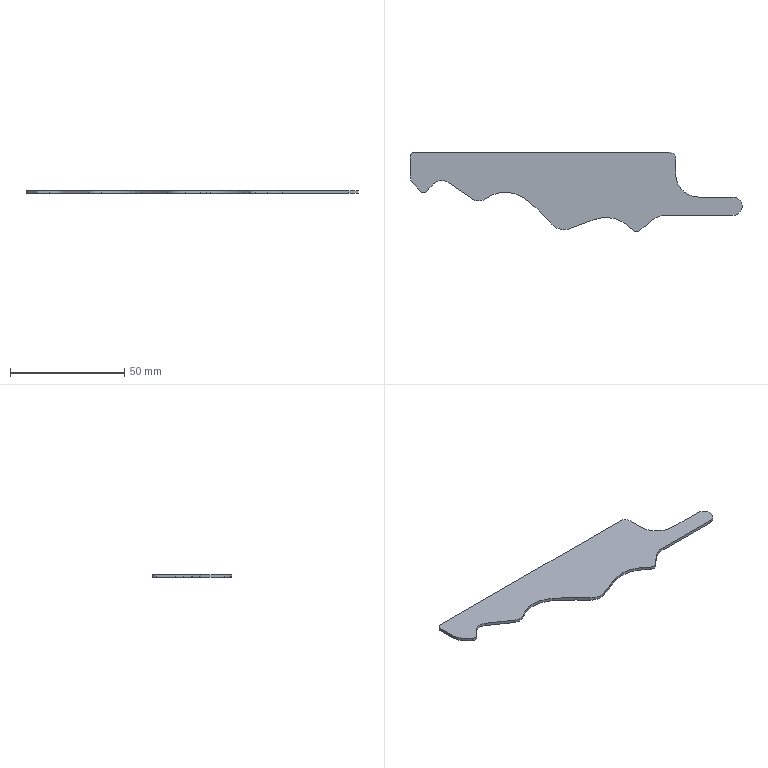Part | STEP file | gslz 2016.10.28-13_id206_x_t | 1 solid | 30 faces | box 145.084 x 34.623 x 1.25 mm | volume 3825 mm3 | plane 15 | cylinder 15 | commonest cylinder face diameters 4 x4 10 x3 20 x2 6 x1 8 x1 14 x1